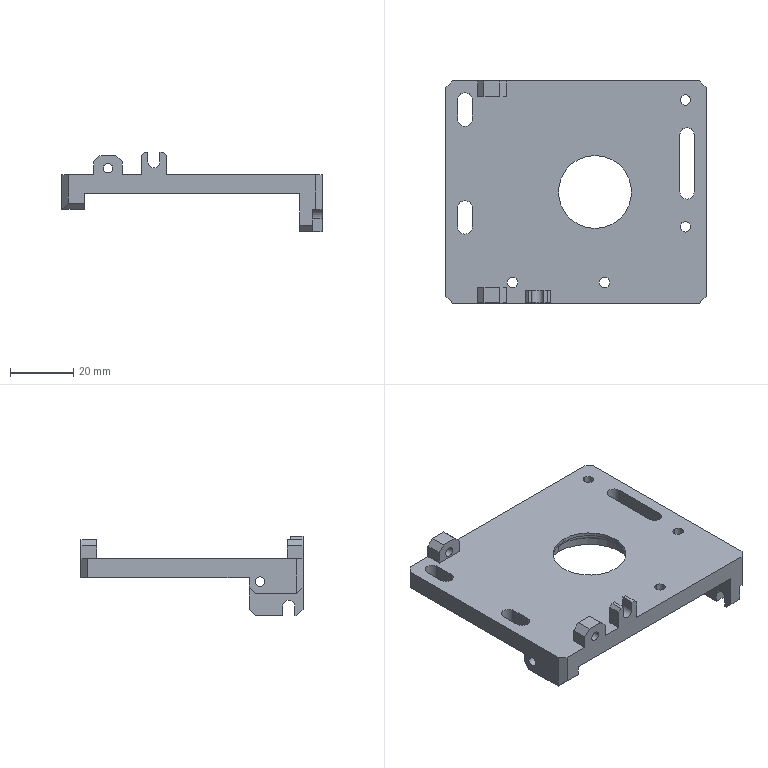Part | 1 solid | 108 faces | box 82 x 70 x 25 mm | volume 31825 mm3 | plane 60 | cylinder 40 | cone 8 | commonest cylinder face diameters 3 x8 3.3 x8 4.6 x6 2 x4 4.5 x3 3.8 x2